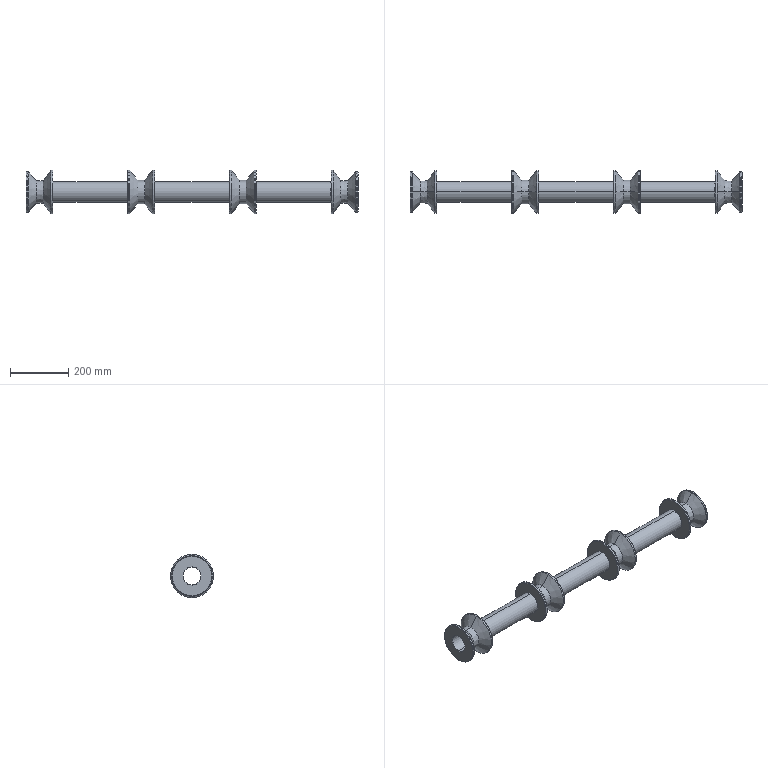Part | SolidWorks | features BaseBody 7 | 7 solids | 134 faces | box 1139 x 148 x 148 mm | volume 3544589 mm3 | cone 52 | cylinder 36 | torus 32 | plane 14 | commonest cylinder face diameters 60 x14 148 x12 72 x6 81.214 x4